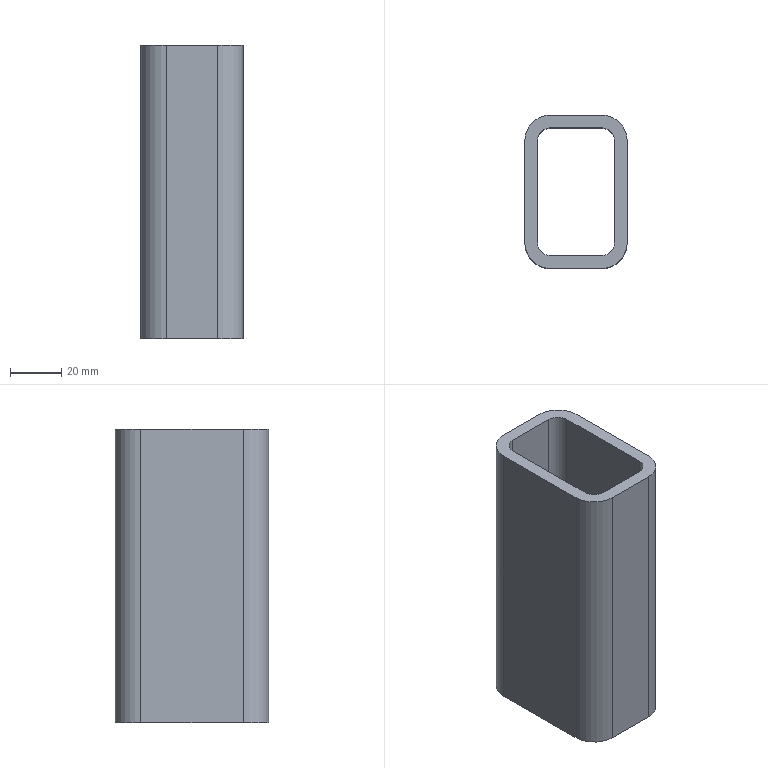Part | STEP file | HL4GD-1.30.113 base frame front support vertical beam--20251212 | 1 solid | 18 faces | box 40 x 60 x 115 mm | volume 96096 mm3 | plane 10 | cylinder 8 | commonest cylinder face diameters 10 x4 20 x4
STEP:
#1=CARTESIAN_POINT('',(0.,0.,0.));
#2=DIRECTION('',(0.,0.,1.));
#3=DIRECTION('',(1.,0.,0.));
#4=AXIS2_PLACEMENT_3D('',#1,#2,#3);
#5=CARTESIAN_POINT('',(2870.,610.,405.));
#6=VERTEX_POINT('',#5);
#7=CARTESIAN_POINT('',(2875.,615.,405.));
#8=VERTEX_POINT('',#7);
#9=CARTESIAN_POINT('',(2875.,610.,405.));
#10=DIRECTION('',(0.,0.,-1.));
#11=DIRECTION('',(0.,1.,0.));
#12=AXIS2_PLACEMENT_3D('',#9,#10,#11);
#13=CIRCLE('',#12,5.);
#14=CARTESIAN_POINT('',(2875.,610.,1349.));
#15=DIRECTION('',(0.,0.,1.));
#16=DIRECTION('',(-1.,0.,0.));
#17=AXIS2_PLACEMENT_3D('',#14,#15,#16);
#18=CYLINDRICAL_SURFACE('',#17,5.);
#19=CARTESIAN_POINT('',(10.996,-944.));
#20=DIRECTION('',(-1.,0.));
#21=VECTOR('',#20,1.);
#22=LINE('',#19,#21);
#23=(GEOMETRIC_REPRESENTATION_CONTEXT(2)PARAMETRIC_REPRESENTATION_CONTEXT()REPRESENTATION_CONTEXT('',''));
#24=DEFINITIONAL_REPRESENTATION('',(#22),#23);
#25=PCURVE('',#18,#24);
#26=CARTESIAN_POINT('',(2885.,1185.,405.));
#27=DIRECTION('',(0.,0.,1.));
#28=DIRECTION('',(0.,1.,0.));
#29=AXIS2_PLACEMENT_3D('',#26,#27,#28);
#30=PLANE('',#29);
#31=CARTESIAN_POINT('',(-570.,10.));
#32=CARTESIAN_POINT('',(-570.,1.34));
#33=CARTESIAN_POINT('',(-577.5,5.67));
#34=CARTESIAN_POINT('',(-585.,10.));
#35=CARTESIAN_POINT('',(-577.5,14.33));
#36=CARTESIAN_POINT('',(-570.,18.66));
#37=CARTESIAN_POINT('',(-570.,10.));
#38=(BOUNDED_CURVE()B_SPLINE_CURVE(2,(#31,#32,#33,#34,#35,#36,#37),.UNSPECIFIED.,.T.,.F.)B_SPLINE_CURVE_WITH_KNOTS((1,2,2,2,2,1),(-2.094,0.,2.094,4.189,6.283,8.378),.UNSPECIFIED.)CURVE()GEOMETRIC_REPRESENTATION_ITEM()RATIONAL_B_SPLINE_CURVE((1.,0.5,1.,0.5,1.,0.5,1.))REPRESENTATION_ITEM(''));
#39=(GEOMETRIC_REPRESENTATION_CONTEXT(2)PARAMETRIC_REPRESENTATION_CONTEXT()REPRESENTATION_CONTEXT('',''));
#40=DEFINITIONAL_REPRESENTATION('',(#38),#39);
#41=PCURVE('',#30,#40);
#42=SURFACE_CURVE('',#13,(#25,#41),.PCURVE_S1.);
#43=EDGE_CURVE('',#6,#8,#42,.T.);
#44=ORIENTED_EDGE('',*,*,#43,.F.);
#45=CARTESIAN_POINT('',(2870.,610.,520.));
#46=VERTEX_POINT('',#45);
#47=CARTESIAN_POINT('',(2870.,610.,1349.));
#48=DIRECTION('',(0.,0.,1.));
#49=VECTOR('',#48,1.);
#50=LINE('',#47,#49);
#51=CARTESIAN_POINT('',(6.283,0.));
#52=DIRECTION('',(0.,1.));
#53=VECTOR('',#52,1.);
#54=LINE('',#51,#53);
#55=(GEOMETRIC_REPRESENTATION_CONTEXT(2)PARAMETRIC_REPRESENTATION_CONTEXT()REPRESENTATION_CONTEXT('',''));
#56=DEFINITIONAL_REPRESENTATION('',(#54),#55);
#57=PCURVE('',#18,#56);
#58=CARTESIAN_POINT('',(2870.,610.,1349.));
#59=DIRECTION('',(1.,0.,0.));
#60=DIRECTION('',(0.,1.,0.));
#61=AXIS2_PLACEMENT_3D('',#58,#59,#60);
#62=PLANE('',#61);
#63=CARTESIAN_POINT('',(0.,0.));
#64=DIRECTION('',(0.,1.));
#65=VECTOR('',#64,1.);
#66=LINE('',#63,#65);
#67=(GEOMETRIC_REPRESENTATION_CONTEXT(2)PARAMETRIC_REPRESENTATION_CONTEXT()REPRESENTATION_CONTEXT('',''));
#68=DEFINITIONAL_REPRESENTATION('',(#66),#67);
#69=PCURVE('',#62,#68);
#70=SURFACE_CURVE('',#50,(#57,#69),.PCURVE_S1.);
#71=EDGE_CURVE('',#6,#46,#70,.T.);
#72=ORIENTED_EDGE('',*,*,#71,.T.);
#73=CARTESIAN_POINT('',(2875.,615.,520.));
#74=VERTEX_POINT('',#73);
#75=CARTESIAN_POINT('',(2875.,610.,520.));
#76=DIRECTION('',(0.,0.,1.));
#77=DIRECTION('',(1.,0.,0.));
#78=AXIS2_PLACEMENT_3D('',#75,#76,#77);
#79=CIRCLE('',#78,5.);
#80=CARTESIAN_POINT('',(3.142,-829.));
#81=DIRECTION('',(1.,0.));
#82=VECTOR('',#81,1.);
#83=LINE('',#80,#82);
#84=(GEOMETRIC_REPRESENTATION_CONTEXT(2)PARAMETRIC_REPRESENTATION_CONTEXT()REPRESENTATION_CONTEXT('',''));
#85=DEFINITIONAL_REPRESENTATION('',(#83),#84);
#86=PCURVE('',#18,#85);
#87=CARTESIAN_POINT('',(2455.,590.,520.));
#88=DIRECTION('',(0.,0.,1.));
#89=DIRECTION('',(1.,0.,0.));
#90=AXIS2_PLACEMENT_3D('',#87,#88,#89);
#91=PLANE('',#90);
#92=CARTESIAN_POINT('',(420.,20.));
#93=DIRECTION('',(1.,0.));
#94=AXIS2_PLACEMENT_2D('',#92,#93);
#95=CIRCLE('',#94,5.);
#96=(GEOMETRIC_REPRESENTATION_CONTEXT(2)PARAMETRIC_REPRESENTATION_CONTEXT()REPRESENTATION_CONTEXT('',''));
#97=DEFINITIONAL_REPRESENTATION('',(#95),#96);
#98=PCURVE('',#91,#97);
#99=SURFACE_CURVE('',#79,(#86,#98),.PCURVE_S1.);
#100=EDGE_CURVE('',#74,#46,#99,.T.);
#101=ORIENTED_EDGE('',*,*,#100,.F.);
#102=CARTESIAN_POINT('',(2875.,615.,1349.));
#103=DIRECTION('',(0.,0.,1.));
#104=VECTOR('',#103,1.);
#105=LINE('',#102,#104);
#106=CARTESIAN_POINT('',(4.712,0.));
#107=DIRECTION('',(0.,1.));
#108=VECTOR('',#107,1.);
#109=LINE('',#106,#108);
#110=(GEOMETRIC_REPRESENTATION_CONTEXT(2)PARAMETRIC_REPRESENTATION_CONTEXT()REPRESENTATION_CONTEXT('',''));
#111=DEFINITIONAL_REPRESENTATION('',(#109),#110);
#112=PCURVE('',#18,#111);
#113=CARTESIAN_POINT('',(2895.,615.,1349.));
#114=DIRECTION('',(0.,-1.,0.));
#115=DIRECTION('',(1.,0.,0.));
#116=AXIS2_PLACEMENT_3D('',#113,#114,#115);
#117=PLANE('',#116);
#118=CARTESIAN_POINT('',(-20.,0.));
#119=DIRECTION('',(0.,1.));
#120=VECTOR('',#119,1.);
#121=LINE('',#118,#120);
#122=(GEOMETRIC_REPRESENTATION_CONTEXT(2)PARAMETRIC_REPRESENTATION_CONTEXT()REPRESENTATION_CONTEXT('',''));
#123=DEFINITIONAL_REPRESENTATION('',(#121),#122);
#124=PCURVE('',#117,#123);
#125=SURFACE_CURVE('',#105,(#112,#124),.PCURVE_S1.);
#126=EDGE_CURVE('',#8,#74,#125,.T.);
#127=ORIENTED_EDGE('',*,*,#126,.F.);
#128=EDGE_LOOP('',(#44,#72,#101,#127));
#129=FACE_BOUND('',#128,.F.);
#130=ADVANCED_FACE('',(#129),#18,.F.);
#131=CARTESIAN_POINT('',(2895.,615.,405.));
#132=VERTEX_POINT('',#131);
#133=CARTESIAN_POINT('',(2895.,615.,520.));
#134=VERTEX_POINT('',#133);
#135=CARTESIAN_POINT('',(2895.,615.,1349.));
#136=DIRECTION('',(0.,0.,1.));
#137=VECTOR('',#136,1.);
#138=LINE('',#135,#137);
#139=CARTESIAN_POINT('',(0.,0.));
#140=DIRECTION('',(0.,1.));
#141=VECTOR('',#140,1.);
#142=LINE('',#139,#141);
#143=(GEOMETRIC_REPRESENTATION_CONTEXT(2)PARAMETRIC_REPRESENTATION_CONTEXT()REPRESENTATION_CONTEXT('',''));
#144=DEFINITIONAL_REPRESENTATION('',(#142),#143);
#145=PCURVE('',#117,#144);
#146=CARTESIAN_POINT('',(2895.,610.,1349.));
#147=DIRECTION('',(0.,0.,1.));
#148=DIRECTION('',(-1.,0.,0.));
#149=AXIS2_PLACEMENT_3D('',#146,#147,#148);
#150=CYLINDRICAL_SURFACE('',#149,5.);
#151=CARTESIAN_POINT('',(4.712,0.));
#152=DIRECTION('',(0.,1.));
#153=VECTOR('',#152,1.);
#154=LINE('',#151,#153);
#155=(GEOMETRIC_REPRESENTATION_CONTEXT(2)PARAMETRIC_REPRESENTATION_CONTEXT()REPRESENTATION_CONTEXT('',''));
#156=DEFINITIONAL_REPRESENTATION('',(#154),#155);
#157=PCURVE('',#150,#156);
#158=SURFACE_CURVE('',#138,(#145,#157),.PCURVE_S1.);
#159=EDGE_CURVE('',#132,#134,#158,.T.);
#160=ORIENTED_EDGE('',*,*,#159,.T.);
#161=CARTESIAN_POINT('',(2895.,615.,520.));
#162=DIRECTION('',(-1.,0.,0.));
#163=VECTOR('',#162,1.);
#164=LINE('',#161,#163);
#165=CARTESIAN_POINT('',(0.,-829.));
#166=DIRECTION('',(-1.,0.));
#167=VECTOR('',#166,1.);
#168=LINE('',#165,#167);
#169=(GEOMETRIC_REPRESENTATION_CONTEXT(2)PARAMETRIC_REPRESENTATION_CONTEXT()REPRESENTATION_CONTEXT('',''));
#170=DEFINITIONAL_REPRESENTATION('',(#168),#169);
#171=PCURVE('',#117,#170);
#172=CARTESIAN_POINT('',(440.,25.));
#173=DIRECTION('',(-1.,0.));
#174=VECTOR('',#173,1.);
#175=LINE('',#172,#174);
#176=(GEOMETRIC_REPRESENTATION_CONTEXT(2)PARAMETRIC_REPRESENTATION_CONTEXT()REPRESENTATION_CONTEXT('',''));
#177=DEFINITIONAL_REPRESENTATION('',(#175),#176);
#178=PCURVE('',#91,#177);
#179=SURFACE_CURVE('',#164,(#171,#178),.PCURVE_S1.);
#180=EDGE_CURVE('',#134,#74,#179,.T.);
#181=ORIENTED_EDGE('',*,*,#180,.T.);
#182=ORIENTED_EDGE('',*,*,#126,.F.);
#183=CARTESIAN_POINT('',(2895.,615.,405.));
#184=DIRECTION('',(1.,0.,0.));
#185=VECTOR('',#184,1.);
#186=LINE('',#183,#185);
#187=CARTESIAN_POINT('',(0.,-944.));
#188=DIRECTION('',(1.,0.));
#189=VECTOR('',#188,1.);
#190=LINE('',#187,#189);
#191=(GEOMETRIC_REPRESENTATION_CONTEXT(2)PARAMETRIC_REPRESENTATION_CONTEXT()REPRESENTATION_CONTEXT('',''));
#192=DEFINITIONAL_REPRESENTATION('',(#190),#191);
#193=PCURVE('',#117,#192);
#194=CARTESIAN_POINT('',(-570.,-10.));
#195=DIRECTION('',(0.,-1.));
#196=VECTOR('',#195,1.);
#197=LINE('',#194,#196);
#198=(GEOMETRIC_REPRESENTATION_CONTEXT(2)PARAMETRIC_REPRESENTATION_CONTEXT()REPRESENTATION_CONTEXT('',''));
#199=DEFINITIONAL_REPRESENTATION('',(#197),#198);
#200=PCURVE('',#30,#199);
#201=SURFACE_CURVE('',#186,(#193,#200),.PCURVE_S1.);
#202=EDGE_CURVE('',#8,#132,#201,.T.);
#203=ORIENTED_EDGE('',*,*,#202,.T.);
#204=EDGE_LOOP('',(#160,#181,#182,#203));
#205=FACE_BOUND('',#204,.T.);
#206=ADVANCED_FACE('',(#205),#117,.T.);
#207=CARTESIAN_POINT('',(2900.,610.,405.));
#208=VERTEX_POINT('',#207);
#209=CARTESIAN_POINT('',(2895.,610.,405.));
#210=DIRECTION('',(0.,0.,1.));
#211=DIRECTION('',(0.,1.,0.));
#212=AXIS2_PLACEMENT_3D('',#209,#210,#211);
#213=CIRCLE('',#212,5.);
#214=CARTESIAN_POINT('',(-1.571,-944.));
#215=DIRECTION('',(1.,0.));
#216=VECTOR('',#215,1.);
#217=LINE('',#214,#216);
#218=(GEOMETRIC_REPRESENTATION_CONTEXT(2)PARAMETRIC_REPRESENTATION_CONTEXT()REPRESENTATION_CONTEXT('',''));
#219=DEFINITIONAL_REPRESENTATION('',(#217),#218);
#220=PCURVE('',#150,#219);
#221=CARTESIAN_POINT('',(-575.,-10.));
#222=DIRECTION('',(1.,0.));
#223=AXIS2_PLACEMENT_2D('',#221,#222);
#224=CIRCLE('',#223,5.);
#225=(GEOMETRIC_REPRESENTATION_CONTEXT(2)PARAMETRIC_REPRESENTATION_CONTEXT()REPRESENTATION_CONTEXT('',''));
#226=DEFINITIONAL_REPRESENTATION('',(#224),#225);
#227=PCURVE('',#30,#226);
#228=SURFACE_CURVE('',#213,(#220,#227),.PCURVE_S1.);
#229=EDGE_CURVE('',#208,#132,#228,.T.);
#230=ORIENTED_EDGE('',*,*,#229,.T.);
#231=ORIENTED_EDGE('',*,*,#159,.T.);
#232=CARTESIAN_POINT('',(2900.,610.,520.));
#233=VERTEX_POINT('',#232);
#234=CARTESIAN_POINT('',(2895.,610.,520.));
#235=DIRECTION('',(0.,0.,1.));
#236=DIRECTION('',(1.,0.,0.));
#237=AXIS2_PLACEMENT_3D('',#234,#235,#236);
#238=CIRCLE('',#237,5.);
#239=CARTESIAN_POINT('',(3.142,-829.));
#240=DIRECTION('',(1.,0.));
#241=VECTOR('',#240,1.);
#242=LINE('',#239,#241);
#243=(GEOMETRIC_REPRESENTATION_CONTEXT(2)PARAMETRIC_REPRESENTATION_CONTEXT()REPRESENTATION_CONTEXT('',''));
#244=DEFINITIONAL_REPRESENTATION('',(#242),#243);
#245=PCURVE('',#150,#244);
#246=CARTESIAN_POINT('',(440.,20.));
#247=DIRECTION('',(1.,0.));
#248=AXIS2_PLACEMENT_2D('',#246,#247);
#249=CIRCLE('',#248,5.);
#250=(GEOMETRIC_REPRESENTATION_CONTEXT(2)PARAMETRIC_REPRESENTATION_CONTEXT()REPRESENTATION_CONTEXT('',''));
#251=DEFINITIONAL_REPRESENTATION('',(#249),#250);
#252=PCURVE('',#91,#251);
#253=SURFACE_CURVE('',#238,(#245,#252),.PCURVE_S1.);
#254=EDGE_CURVE('',#233,#134,#253,.T.);
#255=ORIENTED_EDGE('',*,*,#254,.F.);
#256=CARTESIAN_POINT('',(2900.,610.,1349.));
#257=DIRECTION('',(0.,0.,1.));
#258=VECTOR('',#257,1.);
#259=LINE('',#256,#258);
#260=CARTESIAN_POINT('',(3.142,0.));
#261=DIRECTION('',(0.,1.));
#262=VECTOR('',#261,1.);
#263=LINE('',#260,#262);
#264=(GEOMETRIC_REPRESENTATION_CONTEXT(2)PARAMETRIC_REPRESENTATION_CONTEXT()REPRESENTATION_CONTEXT('',''));
#265=DEFINITIONAL_REPRESENTATION('',(#263),#264);
#266=PCURVE('',#150,#265);
#267=CARTESIAN_POINT('',(2900.,570.,1349.));
#268=DIRECTION('',(-1.,0.,0.));
#269=DIRECTION('',(0.,-1.,0.));
#270=AXIS2_PLACEMENT_3D('',#267,#268,#269);
#271=PLANE('',#270);
#272=CARTESIAN_POINT('',(-40.,0.));
#273=DIRECTION('',(0.,1.));
#274=VECTOR('',#273,1.);
#275=LINE('',#272,#274);
#276=(GEOMETRIC_REPRESENTATION_CONTEXT(2)PARAMETRIC_REPRESENTATION_CONTEXT()REPRESENTATION_CONTEXT('',''));
#277=DEFINITIONAL_REPRESENTATION('',(#275),#276);
#278=PCURVE('',#271,#277);
#279=SURFACE_CURVE('',#259,(#266,#278),.PCURVE_S1.);
#280=EDGE_CURVE('',#208,#233,#279,.T.);
#281=ORIENTED_EDGE('',*,*,#280,.F.);
#282=EDGE_LOOP('',(#230,#231,#255,#281));
#283=FACE_BOUND('',#282,.F.);
#284=ADVANCED_FACE('',(#283),#150,.F.);
#285=CARTESIAN_POINT('',(2900.,570.,405.));
#286=VERTEX_POINT('',#285);
#287=CARTESIAN_POINT('',(2900.,570.,520.));
#288=VERTEX_POINT('',#287);
#289=CARTESIAN_POINT('',(2900.,570.,1349.));
#290=DIRECTION('',(0.,0.,1.));
#291=VECTOR('',#290,1.);
#292=LINE('',#289,#291);
#293=CARTESIAN_POINT('',(0.,0.));
#294=DIRECTION('',(0.,1.));
#295=VECTOR('',#294,1.);
#296=LINE('',#293,#295);
#297=(GEOMETRIC_REPRESENTATION_CONTEXT(2)PARAMETRIC_REPRESENTATION_CONTEXT()REPRESENTATION_CONTEXT('',''));
#298=DEFINITIONAL_REPRESENTATION('',(#296),#297);
#299=PCURVE('',#271,#298);
#300=CARTESIAN_POINT('',(2895.,570.,1349.));
#301=DIRECTION('',(0.,0.,1.));
#302=DIRECTION('',(-1.,0.,0.));
#303=AXIS2_PLACEMENT_3D('',#300,#301,#302);
#304=CYLINDRICAL_SURFACE('',#303,5.);
#305=CARTESIAN_POINT('',(3.142,0.));
#306=DIRECTION('',(0.,1.));
#307=VECTOR('',#306,1.);
#308=LINE('',#305,#307);
#309=(GEOMETRIC_REPRESENTATION_CONTEXT(2)PARAMETRIC_REPRESENTATION_CONTEXT()REPRESENTATION_CONTEXT('',''));
#310=DEFINITIONAL_REPRESENTATION('',(#308),#309);
#311=PCURVE('',#304,#310);
#312=SURFACE_CURVE('',#292,(#299,#311),.PCURVE_S1.);
#313=EDGE_CURVE('',#286,#288,#312,.T.);
#314=ORIENTED_EDGE('',*,*,#313,.T.);
#315=CARTESIAN_POINT('',(2900.,570.,520.));
#316=DIRECTION('',(0.,1.,0.));
#317=VECTOR('',#316,1.);
#318=LINE('',#315,#317);
#319=CARTESIAN_POINT('',(0.,-829.));
#320=DIRECTION('',(-1.,0.));
#321=VECTOR('',#320,1.);
#322=LINE('',#319,#321);
#323=(GEOMETRIC_REPRESENTATION_CONTEXT(2)PARAMETRIC_REPRESENTATION_CONTEXT()REPRESENTATION_CONTEXT('',''));
#324=DEFINITIONAL_REPRESENTATION('',(#322),#323);
#325=PCURVE('',#271,#324);
#326=CARTESIAN_POINT('',(445.,-20.));
#327=DIRECTION('',(0.,1.));
#328=VECTOR('',#327,1.);
#329=LINE('',#326,#328);
#330=(GEOMETRIC_REPRESENTATION_CONTEXT(2)PARAMETRIC_REPRESENTATION_CONTEXT()REPRESENTATION_CONTEXT('',''));
#331=DEFINITIONAL_REPRESENTATION('',(#329),#330);
#332=PCURVE('',#91,#331);
#333=SURFACE_CURVE('',#318,(#325,#332),.PCURVE_S1.);
#334=EDGE_CURVE('',#288,#233,#333,.T.);
#335=ORIENTED_EDGE('',*,*,#334,.T.);
#336=ORIENTED_EDGE('',*,*,#280,.F.);
#337=CARTESIAN_POINT('',(2900.,570.,405.));
#338=DIRECTION('',(0.,1.,0.));
#339=VECTOR('',#338,1.);
#340=LINE('',#337,#339);
#341=CARTESIAN_POINT('',(0.,-944.));
#342=DIRECTION('',(-1.,0.));
#343=VECTOR('',#342,1.);
#344=LINE('',#341,#343);
#345=(GEOMETRIC_REPRESENTATION_CONTEXT(2)PARAMETRIC_REPRESENTATION_CONTEXT()REPRESENTATION_CONTEXT('',''));
#346=DEFINITIONAL_REPRESENTATION('',(#344),#345);
#347=PCURVE('',#271,#346);
#348=CARTESIAN_POINT('',(-615.,-15.));
#349=DIRECTION('',(1.,0.));
#350=VECTOR('',#349,1.);
#351=LINE('',#348,#350);
#352=(GEOMETRIC_REPRESENTATION_CONTEXT(2)PARAMETRIC_REPRESENTATION_CONTEXT()REPRESENTATION_CONTEXT('',''));
#353=DEFINITIONAL_REPRESENTATION('',(#351),#352);
#354=PCURVE('',#30,#353);
#355=SURFACE_CURVE('',#340,(#347,#354),.PCURVE_S1.);
#356=EDGE_CURVE('',#286,#208,#355,.T.);
#357=ORIENTED_EDGE('',*,*,#356,.F.);
#358=EDGE_LOOP('',(#314,#335,#336,#357));
#359=FACE_BOUND('',#358,.T.);
#360=ADVANCED_FACE('',(#359),#271,.T.);
#361=CARTESIAN_POINT('',(2895.,565.,405.));
#362=VERTEX_POINT('',#361);
#363=CARTESIAN_POINT('',(2895.,570.,405.));
#364=DIRECTION('',(0.,0.,1.));
#365=DIRECTION('',(0.,1.,0.));
#366=AXIS2_PLACEMENT_3D('',#363,#364,#365);
#367=CIRCLE('',#366,5.);
#368=CARTESIAN_POINT('',(-1.571,-944.));
#369=DIRECTION('',(1.,0.));
#370=VECTOR('',#369,1.);
#371=LINE('',#368,#370);
#372=(GEOMETRIC_REPRESENTATION_CONTEXT(2)PARAMETRIC_REPRESENTATION_CONTEXT()REPRESENTATION_CONTEXT('',''));
#373=DEFINITIONAL_REPRESENTATION('',(#371),#372);
#374=PCURVE('',#304,#373);
#375=CARTESIAN_POINT('',(-615.,-10.));
#376=DIRECTION('',(1.,0.));
#377=AXIS2_PLACEMENT_2D('',#375,#376);
#378=CIRCLE('',#377,5.);
#379=(GEOMETRIC_REPRESENTATION_CONTEXT(2)PARAMETRIC_REPRESENTATION_CONTEXT()REPRESENTATION_CONTEXT('',''));
#380=DEFINITIONAL_REPRESENTATION('',(#378),#379);
#381=PCURVE('',#30,#380);
#382=SURFACE_CURVE('',#367,(#374,#381),.PCURVE_S1.);
#383=EDGE_CURVE('',#362,#286,#382,.T.);
#384=ORIENTED_EDGE('',*,*,#383,.T.);
#385=ORIENTED_EDGE('',*,*,#313,.T.);
#386=CARTESIAN_POINT('',(2895.,565.,520.));
#387=VERTEX_POINT('',#386);
#388=CARTESIAN_POINT('',(2895.,570.,520.));
#389=DIRECTION('',(0.,0.,1.));
#390=DIRECTION('',(1.,0.,0.));
#391=AXIS2_PLACEMENT_3D('',#388,#389,#390);
#392=CIRCLE('',#391,5.);
#393=CARTESIAN_POINT('',(-3.142,-829.));
#394=DIRECTION('',(1.,0.));
#395=VECTOR('',#394,1.);
#396=LINE('',#393,#395);
#397=(GEOMETRIC_REPRESENTATION_CONTEXT(2)PARAMETRIC_REPRESENTATION_CONTEXT()REPRESENTATION_CONTEXT('',''));
#398=DEFINITIONAL_REPRESENTATION('',(#396),#397);
#399=PCURVE('',#304,#398);
#400=CARTESIAN_POINT('',(440.,-20.));
#401=DIRECTION('',(1.,0.));
#402=AXIS2_PLACEMENT_2D('',#400,#401);
#403=CIRCLE('',#402,5.);
#404=(GEOMETRIC_REPRESENTATION_CONTEXT(2)PARAMETRIC_REPRESENTATION_CONTEXT()REPRESENTATION_CONTEXT('',''));
#405=DEFINITIONAL_REPRESENTATION('',(#403),#404);
#406=PCURVE('',#91,#405);
#407=SURFACE_CURVE('',#392,(#399,#406),.PCURVE_S1.);
#408=EDGE_CURVE('',#387,#288,#407,.T.);
#409=ORIENTED_EDGE('',*,*,#408,.F.);
#410=CARTESIAN_POINT('',(2895.,565.,1349.));
#411=DIRECTION('',(0.,0.,1.));
#412=VECTOR('',#411,1.);
#413=LINE('',#410,#412);
#414=CARTESIAN_POINT('',(1.571,0.));
#415=DIRECTION('',(0.,1.));
#416=VECTOR('',#415,1.);
#417=LINE('',#414,#416);
#418=(GEOMETRIC_REPRESENTATION_CONTEXT(2)PARAMETRIC_REPRESENTATION_CONTEXT()REPRESENTATION_CONTEXT('',''));
#419=DEFINITIONAL_REPRESENTATION('',(#417),#418);
#420=PCURVE('',#304,#419);
#421=CARTESIAN_POINT('',(2875.,565.,1349.));
#422=DIRECTION('',(0.,1.,0.));
#423=DIRECTION('',(-1.,0.,0.));
#424=AXIS2_PLACEMENT_3D('',#421,#422,#423);
#425=PLANE('',#424);
#426=CARTESIAN_POINT('',(-20.,0.));
#427=DIRECTION('',(0.,1.));
#428=VECTOR('',#427,1.);
#429=LINE('',#426,#428);
#430=(GEOMETRIC_REPRESENTATION_CONTEXT(2)PARAMETRIC_REPRESENTATION_CONTEXT()REPRESENTATION_CONTEXT('',''));
#431=DEFINITIONAL_REPRESENTATION('',(#429),#430);
#432=PCURVE('',#425,#431);
#433=SURFACE_CURVE('',#413,(#420,#432),.PCURVE_S1.);
#434=EDGE_CURVE('',#362,#387,#433,.T.);
#435=ORIENTED_EDGE('',*,*,#434,.F.);
#436=EDGE_LOOP('',(#384,#385,#409,#435));
#437=FACE_BOUND('',#436,.F.);
#438=ADVANCED_FACE('',(#437),#304,.F.);
#439=CARTESIAN_POINT('',(2875.,565.,405.));
#440=VERTEX_POINT('',#439);
#441=CARTESIAN_POINT('',(2875.,565.,520.));
#442=VERTEX_POINT('',#441);
#443=CARTESIAN_POINT('',(2875.,565.,1349.));
#444=DIRECTION('',(0.,0.,1.));
#445=VECTOR('',#444,1.);
#446=LINE('',#443,#445);
#447=CARTESIAN_POINT('',(0.,0.));
#448=DIRECTION('',(0.,1.));
#449=VECTOR('',#448,1.);
#450=LINE('',#447,#449);
#451=(GEOMETRIC_REPRESENTATION_CONTEXT(2)PARAMETRIC_REPRESENTATION_CONTEXT()REPRESENTATION_CONTEXT('',''));
#452=DEFINITIONAL_REPRESENTATION('',(#450),#451);
#453=PCURVE('',#425,#452);
#454=CARTESIAN_POINT('',(2875.,570.,1349.));
#455=DIRECTION('',(0.,0.,1.));
#456=DIRECTION('',(-1.,0.,0.));
#457=AXIS2_PLACEMENT_3D('',#454,#455,#456);
#458=CYLINDRICAL_SURFACE('',#457,5.);
#459=CARTESIAN_POINT('',(1.571,0.));
#460=DIRECTION('',(0.,1.));
#461=VECTOR('',#460,1.);
#462=LINE('',#459,#461);
#463=(GEOMETRIC_REPRESENTATION_CONTEXT(2)PARAMETRIC_REPRESENTATION_CONTEXT()REPRESENTATION_CONTEXT('',''));
#464=DEFINITIONAL_REPRESENTATION('',(#462),#463);
#465=PCURVE('',#458,#464);
#466=SURFACE_CURVE('',#446,(#453,#465),.PCURVE_S1.);
#467=EDGE_CURVE('',#440,#442,#466,.T.);
#468=ORIENTED_EDGE('',*,*,#467,.T.);
#469=CARTESIAN_POINT('',(2875.,565.,520.));
#470=DIRECTION('',(1.,0.,0.));
#471=VECTOR('',#470,1.);
#472=LINE('',#469,#471);
#473=CARTESIAN_POINT('',(0.,-829.));
#474=DIRECTION('',(-1.,0.));
#475=VECTOR('',#474,1.);
#476=LINE('',#473,#475);
#477=(GEOMETRIC_REPRESENTATION_CONTEXT(2)PARAMETRIC_REPRESENTATION_CONTEXT()REPRESENTATION_CONTEXT('',''));
#478=DEFINITIONAL_REPRESENTATION('',(#476),#477);
#479=PCURVE('',#425,#478);
#480=CARTESIAN_POINT('',(420.,-25.));
#481=DIRECTION('',(1.,0.));
#482=VECTOR('',#481,1.);
#483=LINE('',#480,#482);
#484=(GEOMETRIC_REPRESENTATION_CONTEXT(2)PARAMETRIC_REPRESENTATION_CONTEXT()REPRESENTATION_CONTEXT('',''));
#485=DEFINITIONAL_REPRESENTATION('',(#483),#484);
#486=PCURVE('',#91,#485);
#487=SURFACE_CURVE('',#472,(#479,#486),.PCURVE_S1.);
#488=EDGE_CURVE('',#442,#387,#487,.T.);
#489=ORIENTED_EDGE('',*,*,#488,.T.);
#490=ORIENTED_EDGE('',*,*,#434,.F.);
#491=CARTESIAN_POINT('',(2875.,565.,405.));
#492=DIRECTION('',(1.,0.,0.));
#493=VECTOR('',#492,1.);
#494=LINE('',#491,#493);
#495=CARTESIAN_POINT('',(0.,-944.));
#496=DIRECTION('',(-1.,0.));
#497=VECTOR('',#496,1.);
#498=LINE('',#495,#497);
#499=(GEOMETRIC_REPRESENTATION_CONTEXT(2)PARAMETRIC_REPRESENTATION_CONTEXT()REPRESENTATION_CONTEXT('',''));
#500=DEFINITIONAL_REPRESENTATION('',(#498),#499);
#501=PCURVE('',#425,#500);
#502=CARTESIAN_POINT('',(-620.,10.));
#503=DIRECTION('',(0.,-1.));
#504=VECTOR('',#503,1.);
#505=LINE('',#502,#504);
#506=(GEOMETRIC_REPRESENTATION_CONTEXT(2)PARAMETRIC_REPRESENTATION_CONTEXT()REPRESENTATION_CONTEXT('',''));
#507=DEFINITIONAL_REPRESENTATION('',(#505),#506);
#508=PCURVE('',#30,#507);
#509=SURFACE_CURVE('',#494,(#501,#508),.PCURVE_S1.);
#510=EDGE_CURVE('',#440,#362,#509,.T.);
#511=ORIENTED_EDGE('',*,*,#510,.F.);
#512=EDGE_LOOP('',(#468,#489,#490,#511));
#513=FACE_BOUND('',#512,.T.);
#514=ADVANCED_FACE('',(#513),#425,.T.);
#515=CARTESIAN_POINT('',(2870.,570.,405.));
#516=VERTEX_POINT('',#515);
#517=CARTESIAN_POINT('',(2875.,570.,405.));
#518=DIRECTION('',(0.,0.,-1.));
#519=DIRECTION('',(0.,1.,0.));
#520=AXIS2_PLACEMENT_3D('',#517,#518,#519);
#521=CIRCLE('',#520,5.);
#522=CARTESIAN_POINT('',(4.712,-944.));
#523=DIRECTION('',(-1.,0.));
#524=VECTOR('',#523,1.);
#525=LINE('',#522,#524);
#526=(GEOMETRIC_REPRESENTATION_CONTEXT(2)PARAMETRIC_REPRESENTATION_CONTEXT()REPRESENTATION_CONTEXT('',''));
#527=DEFINITIONAL_REPRESENTATION('',(#525),#526);
#528=PCURVE('',#458,#527);
#529=CARTESIAN_POINT('',(-610.,10.));
#530=CARTESIAN_POINT('',(-610.,1.34));
#531=CARTESIAN_POINT('',(-617.5,5.67));
#532=CARTESIAN_POINT('',(-625.,10.));
#533=CARTESIAN_POINT('',(-617.5,14.33));
#534=CARTESIAN_POINT('',(-610.,18.66));
#535=CARTESIAN_POINT('',(-610.,10.));
#536=(BOUNDED_CURVE()B_SPLINE_CURVE(2,(#529,#530,#531,#532,#533,#534,#535),.UNSPECIFIED.,.T.,.F.)B_SPLINE_CURVE_WITH_KNOTS((1,2,2,2,2,1),(-2.094,0.,2.094,4.189,6.283,8.378),.UNSPECIFIED.)CURVE()GEOMETRIC_REPRESENTATION_ITEM()RATIONAL_B_SPLINE_CURVE((1.,0.5,1.,0.5,1.,0.5,1.))REPRESENTATION_ITEM(''));
#537=(GEOMETRIC_REPRESENTATION_CONTEXT(2)PARAMETRIC_REPRESENTATION_CONTEXT()REPRESENTATION_CONTEXT('',''));
#538=DEFINITIONAL_REPRESENTATION('',(#536),#537);
#539=PCURVE('',#30,#538);
#540=SURFACE_CURVE('',#521,(#528,#539),.PCURVE_S1.);
#541=EDGE_CURVE('',#440,#516,#540,.T.);
#542=ORIENTED_EDGE('',*,*,#541,.F.);
#543=ORIENTED_EDGE('',*,*,#467,.T.);
#544=CARTESIAN_POINT('',(2870.,570.,520.));
#545=VERTEX_POINT('',#544);
#546=CARTESIAN_POINT('',(2875.,570.,520.));
#547=DIRECTION('',(0.,0.,1.));
#548=DIRECTION('',(1.,0.,0.));
#549=AXIS2_PLACEMENT_3D('',#546,#547,#548);
#550=CIRCLE('',#549,5.);
#551=CARTESIAN_POINT('',(-3.142,-829.));
#552=DIRECTION('',(1.,0.));
#553=VECTOR('',#552,1.);
#554=LINE('',#551,#553);
#555=(GEOMETRIC_REPRESENTATION_CONTEXT(2)PARAMETRIC_REPRESENTATION_CONTEXT()REPRESENTATION_CONTEXT('',''));
#556=DEFINITIONAL_REPRESENTATION('',(#554),#555);
#557=PCURVE('',#458,#556);
#558=CARTESIAN_POINT('',(420.,-20.));
#559=DIRECTION('',(1.,0.));
#560=AXIS2_PLACEMENT_2D('',#558,#559);
#561=CIRCLE('',#560,5.);
#562=(GEOMETRIC_REPRESENTATION_CONTEXT(2)PARAMETRIC_REPRESENTATION_CONTEXT()REPRESENTATION_CONTEXT('',''));
#563=DEFINITIONAL_REPRESENTATION('',(#561),#562);
#564=PCURVE('',#91,#563);
#565=SURFACE_CURVE('',#550,(#557,#564),.PCURVE_S1.);
#566=EDGE_CURVE('',#545,#442,#565,.T.);
#567=ORIENTED_EDGE('',*,*,#566,.F.);
#568=CARTESIAN_POINT('',(2870.,570.,1349.));
#569=DIRECTION('',(0.,0.,1.));
#570=VECTOR('',#569,1.);
#571=LINE('',#568,#570);
#572=CARTESIAN_POINT('',(0.,0.));
#573=DIRECTION('',(0.,1.));
#574=VECTOR('',#573,1.);
#575=LINE('',#572,#574);
#576=(GEOMETRIC_REPRESENTATION_CONTEXT(2)PARAMETRIC_REPRESENTATION_CONTEXT()REPRESENTATION_CONTEXT('',''));
#577=DEFINITIONAL_REPRESENTATION('',(#575),#576);
#578=PCURVE('',#458,#577);
#579=CARTESIAN_POINT('',(-40.,0.));
#580=DIRECTION('',(0.,1.));
#581=VECTOR('',#580,1.);
#582=LINE('',#579,#581);
#583=(GEOMETRIC_REPRESENTATION_CONTEXT(2)PARAMETRIC_REPRESENTATION_CONTEXT()REPRESENTATION_CONTEXT('',''));
#584=DEFINITIONAL_REPRESENTATION('',(#582),#583);
#585=PCURVE('',#62,#584);
#586=SURFACE_CURVE('',#571,(#578,#585),.PCURVE_S1.);
#587=EDGE_CURVE('',#516,#545,#586,.T.);
#588=ORIENTED_EDGE('',*,*,#587,.F.);
#589=EDGE_LOOP('',(#542,#543,#567,#588));
#590=FACE_BOUND('',#589,.F.);
#591=ADVANCED_FACE('',(#590),#458,.F.);
#592=CARTESIAN_POINT('',(2905.,610.,405.));
#593=VERTEX_POINT('',#592);
#594=CARTESIAN_POINT('',(2905.,610.,520.));
#595=VERTEX_POINT('',#594);
#596=CARTESIAN_POINT('',(2905.,610.,1349.));
#597=DIRECTION('',(0.,0.,1.));
#598=VECTOR('',#597,1.);
#599=LINE('',#596,#598);
#600=CARTESIAN_POINT('',(2905.,570.,1349.));
#601=DIRECTION('',(-1.,0.,0.));
#602=DIRECTION('',(0.,-1.,0.));
#603=AXIS2_PLACEMENT_3D('',#600,#601,#602);
#604=PLANE('',#603);
#605=CARTESIAN_POINT('',(-40.,0.));
#606=DIRECTION('',(0.,1.));
#607=VECTOR('',#606,1.);
#608=LINE('',#605,#607);
#609=(GEOMETRIC_REPRESENTATION_CONTEXT(2)PARAMETRIC_REPRESENTATION_CONTEXT()REPRESENTATION_CONTEXT('',''));
#610=DEFINITIONAL_REPRESENTATION('',(#608),#609);
#611=PCURVE('',#604,#610);
#612=CARTESIAN_POINT('',(2895.,610.,1349.));
#613=DIRECTION('',(0.,0.,1.));
#614=DIRECTION('',(-1.,0.,0.));
#615=AXIS2_PLACEMENT_3D('',#612,#613,#614);
#616=CYLINDRICAL_SURFACE('',#615,10.);
#617=CARTESIAN_POINT('',(3.142,0.));
#618=DIRECTION('',(0.,1.));
#619=VECTOR('',#618,1.);
#620=LINE('',#617,#619);
#621=(GEOMETRIC_REPRESENTATION_CONTEXT(2)PARAMETRIC_REPRESENTATION_CONTEXT()REPRESENTATION_CONTEXT('',''));
#622=DEFINITIONAL_REPRESENTATION('',(#620),#621);
#623=PCURVE('',#616,#622);
#624=SURFACE_CURVE('',#599,(#611,#623),.PCURVE_S1.);
#625=EDGE_CURVE('',#593,#595,#624,.T.);
#626=ORIENTED_EDGE('',*,*,#625,.T.);
#627=CARTESIAN_POINT('',(2905.,570.,520.));
#628=VERTEX_POINT('',#627);
#629=CARTESIAN_POINT('',(2905.,570.,520.));
#630=DIRECTION('',(0.,-1.,0.));
#631=VECTOR('',#630,1.);
#632=LINE('',#629,#631);
#633=CARTESIAN_POINT('',(0.,-829.));
#634=DIRECTION('',(1.,0.));
#635=VECTOR('',#634,1.);
#636=LINE('',#633,#635);
#637=(GEOMETRIC_REPRESENTATION_CONTEXT(2)PARAMETRIC_REPRESENTATION_CONTEXT()REPRESENTATION_CONTEXT('',''));
#638=DEFINITIONAL_REPRESENTATION('',(#636),#637);
#639=PCURVE('',#604,#638);
#640=CARTESIAN_POINT('',(450.,-20.));
#641=DIRECTION('',(0.,-1.));
#642=VECTOR('',#641,1.);
#643=LINE('',#640,#642);
#644=(GEOMETRIC_REPRESENTATION_CONTEXT(2)PARAMETRIC_REPRESENTATION_CONTEXT()REPRESENTATION_CONTEXT('',''));
#645=DEFINITIONAL_REPRESENTATION('',(#643),#644);
#646=PCURVE('',#91,#645);
#647=SURFACE_CURVE('',#632,(#639,#646),.PCURVE_S1.);
#648=EDGE_CURVE('',#595,#628,#647,.T.);
#649=ORIENTED_EDGE('',*,*,#648,.T.);
#650=CARTESIAN_POINT('',(2905.,570.,405.));
#651=VERTEX_POINT('',#650);
#652=CARTESIAN_POINT('',(2905.,570.,1349.));
#653=DIRECTION('',(0.,0.,1.));
#654=VECTOR('',#653,1.);
#655=LINE('',#652,#654);
#656=CARTESIAN_POINT('',(0.,0.));
#657=DIRECTION('',(0.,1.));
#658=VECTOR('',#657,1.);
#659=LINE('',#656,#658);
#660=(GEOMETRIC_REPRESENTATION_CONTEXT(2)PARAMETRIC_REPRESENTATION_CONTEXT()REPRESENTATION_CONTEXT('',''));
#661=DEFINITIONAL_REPRESENTATION('',(#659),#660);
#662=PCURVE('',#604,#661);
#663=CARTESIAN_POINT('',(2895.,570.,1349.));
#664=DIRECTION('',(0.,0.,1.));
#665=DIRECTION('',(-1.,0.,0.));
#666=AXIS2_PLACEMENT_3D('',#663,#664,#665);
#667=CYLINDRICAL_SURFACE('',#666,10.);
#668=CARTESIAN_POINT('',(3.142,0.));
#669=DIRECTION('',(0.,1.));
#670=VECTOR('',#669,1.);
#671=LINE('',#668,#670);
#672=(GEOMETRIC_REPRESENTATION_CONTEXT(2)PARAMETRIC_REPRESENTATION_CONTEXT()REPRESENTATION_CONTEXT('',''));
#673=DEFINITIONAL_REPRESENTATION('',(#671),#672);
#674=PCURVE('',#667,#673);
#675=SURFACE_CURVE('',#655,(#662,#674),.PCURVE_S1.);
#676=EDGE_CURVE('',#651,#628,#675,.T.);
#677=ORIENTED_EDGE('',*,*,#676,.F.);
#678=CARTESIAN_POINT('',(2905.,570.,405.));
#679=DIRECTION('',(0.,1.,0.));
#680=VECTOR('',#679,1.);
#681=LINE('',#678,#680);
#682=CARTESIAN_POINT('',(0.,-944.));
#683=DIRECTION('',(-1.,0.));
#684=VECTOR('',#683,1.);
#685=LINE('',#682,#684);
#686=(GEOMETRIC_REPRESENTATION_CONTEXT(2)PARAMETRIC_REPRESENTATION_CONTEXT()REPRESENTATION_CONTEXT('',''));
#687=DEFINITIONAL_REPRESENTATION('',(#685),#686);
#688=PCURVE('',#604,#687);
#689=CARTESIAN_POINT('',(-615.,-20.));
#690=DIRECTION('',(1.,0.));
#691=VECTOR('',#690,1.);
#692=LINE('',#689,#691);
#693=(GEOMETRIC_REPRESENTATION_CONTEXT(2)PARAMETRIC_REPRESENTATION_CONTEXT()REPRESENTATION_CONTEXT('',''));
#694=DEFINITIONAL_REPRESENTATION('',(#692),#693);
#695=PCURVE('',#30,#694);
#696=SURFACE_CURVE('',#681,(#688,#695),.PCURVE_S1.);
#697=EDGE_CURVE('',#651,#593,#696,.T.);
#698=ORIENTED_EDGE('',*,*,#697,.T.);
#699=EDGE_LOOP('',(#626,#649,#677,#698));
#700=FACE_BOUND('',#699,.T.);
#701=ADVANCED_FACE('',(#700),#604,.F.);
#702=CARTESIAN_POINT('',(2895.,620.,405.));
#703=VERTEX_POINT('',#702);
#704=CARTESIAN_POINT('',(2895.,620.,520.));
#705=VERTEX_POINT('',#704);
#706=CARTESIAN_POINT('',(2895.,620.,1349.));
#707=DIRECTION('',(0.,0.,1.));
#708=VECTOR('',#707,1.);
#709=LINE('',#706,#708);
#710=CARTESIAN_POINT('',(4.712,0.));
#711=DIRECTION('',(0.,1.));
#712=VECTOR('',#711,1.);
#713=LINE('',#710,#712);
#714=(GEOMETRIC_REPRESENTATION_CONTEXT(2)PARAMETRIC_REPRESENTATION_CONTEXT()REPRESENTATION_CONTEXT('',''));
#715=DEFINITIONAL_REPRESENTATION('',(#713),#714);
#716=PCURVE('',#616,#715);
#717=CARTESIAN_POINT('',(2895.,620.,1349.));
#718=DIRECTION('',(0.,-1.,0.));
#719=DIRECTION('',(1.,0.,0.));
#720=AXIS2_PLACEMENT_3D('',#717,#718,#719);
#721=PLANE('',#720);
#722=CARTESIAN_POINT('',(0.,0.));
#723=DIRECTION('',(0.,1.));
#724=VECTOR('',#723,1.);
#725=LINE('',#722,#724);
#726=(GEOMETRIC_REPRESENTATION_CONTEXT(2)PARAMETRIC_REPRESENTATION_CONTEXT()REPRESENTATION_CONTEXT('',''));
#727=DEFINITIONAL_REPRESENTATION('',(#725),#726);
#728=PCURVE('',#721,#727);
#729=SURFACE_CURVE('',#709,(#716,#728),.PCURVE_S1.);
#730=EDGE_CURVE('',#703,#705,#729,.T.);
#731=ORIENTED_EDGE('',*,*,#730,.T.);
#732=CARTESIAN_POINT('',(2895.,610.,520.));
#733=DIRECTION('',(0.,0.,-1.));
#734=DIRECTION('',(1.,0.,0.));
#735=AXIS2_PLACEMENT_3D('',#732,#733,#734);
#736=CIRCLE('',#735,10.);
#737=CARTESIAN_POINT('',(9.425,-829.));
#738=DIRECTION('',(-1.,0.));
#739=VECTOR('',#738,1.);
#740=LINE('',#737,#739);
#741=(GEOMETRIC_REPRESENTATION_CONTEXT(2)PARAMETRIC_REPRESENTATION_CONTEXT()REPRESENTATION_CONTEXT('',''));
#742=DEFINITIONAL_REPRESENTATION('',(#740),#741);
#743=PCURVE('',#616,#742);
#744=CARTESIAN_POINT('',(450.,20.));
#745=CARTESIAN_POINT('',(450.,2.679));
#746=CARTESIAN_POINT('',(435.,11.34));
#747=CARTESIAN_POINT('',(420.,20.));
#748=CARTESIAN_POINT('',(435.,28.66));
#749=CARTESIAN_POINT('',(450.,37.321));
#750=CARTESIAN_POINT('',(450.,20.));
#751=(BOUNDED_CURVE()B_SPLINE_CURVE(2,(#744,#745,#746,#747,#748,#749,#750),.UNSPECIFIED.,.T.,.F.)B_SPLINE_CURVE_WITH_KNOTS((1,2,2,2,2,1),(-2.094,0.,2.094,4.189,6.283,8.378),.UNSPECIFIED.)CURVE()GEOMETRIC_REPRESENTATION_ITEM()RATIONAL_B_SPLINE_CURVE((1.,0.5,1.,0.5,1.,0.5,1.))REPRESENTATION_ITEM(''));
#752=(GEOMETRIC_REPRESENTATION_CONTEXT(2)PARAMETRIC_REPRESENTATION_CONTEXT()REPRESENTATION_CONTEXT('',''));
#753=DEFINITIONAL_REPRESENTATION('',(#751),#752);
#754=PCURVE('',#91,#753);
#755=SURFACE_CURVE('',#736,(#743,#754),.PCURVE_S1.);
#756=EDGE_CURVE('',#705,#595,#755,.T.);
#757=ORIENTED_EDGE('',*,*,#756,.T.);
#758=ORIENTED_EDGE('',*,*,#625,.F.);
#759=CARTESIAN_POINT('',(2895.,610.,405.));
#760=DIRECTION('',(0.,0.,1.));
#761=DIRECTION('',(0.,1.,0.));
#762=AXIS2_PLACEMENT_3D('',#759,#760,#761);
#763=CIRCLE('',#762,10.);
#764=CARTESIAN_POINT('',(-1.571,-944.));
#765=DIRECTION('',(1.,0.));
#766=VECTOR('',#765,1.);
#767=LINE('',#764,#766);
#768=(GEOMETRIC_REPRESENTATION_CONTEXT(2)PARAMETRIC_REPRESENTATION_CONTEXT()REPRESENTATION_CONTEXT('',''));
#769=DEFINITIONAL_REPRESENTATION('',(#767),#768);
#770=PCURVE('',#616,#769);
#771=CARTESIAN_POINT('',(-575.,-10.));
#772=DIRECTION('',(1.,0.));
#773=AXIS2_PLACEMENT_2D('',#771,#772);
#774=CIRCLE('',#773,10.);
#775=(GEOMETRIC_REPRESENTATION_CONTEXT(2)PARAMETRIC_REPRESENTATION_CONTEXT()REPRESENTATION_CONTEXT('',''));
#776=DEFINITIONAL_REPRESENTATION('',(#774),#775);
#777=PCURVE('',#30,#776);
#778=SURFACE_CURVE('',#763,(#770,#777),.PCURVE_S1.);
#779=EDGE_CURVE('',#593,#703,#778,.T.);
#780=ORIENTED_EDGE('',*,*,#779,.T.);
#781=EDGE_LOOP('',(#731,#757,#758,#780));
#782=FACE_BOUND('',#781,.T.);
#783=ADVANCED_FACE('',(#782),#616,.T.);
#784=CARTESIAN_POINT('',(2875.,620.,405.));
#785=VERTEX_POINT('',#784);
#786=CARTESIAN_POINT('',(2875.,620.,520.));
#787=VERTEX_POINT('',#786);
#788=CARTESIAN_POINT('',(2875.,620.,1349.));
#789=DIRECTION('',(0.,0.,1.));
#790=VECTOR('',#789,1.);
#791=LINE('',#788,#790);
#792=CARTESIAN_POINT('',(-20.,0.));
#793=DIRECTION('',(0.,1.));
#794=VECTOR('',#793,1.);
#795=LINE('',#792,#794);
#796=(GEOMETRIC_REPRESENTATION_CONTEXT(2)PARAMETRIC_REPRESENTATION_CONTEXT()REPRESENTATION_CONTEXT('',''));
#797=DEFINITIONAL_REPRESENTATION('',(#795),#796);
#798=PCURVE('',#721,#797);
#799=CARTESIAN_POINT('',(2875.,610.,1349.));
#800=DIRECTION('',(0.,0.,1.));
#801=DIRECTION('',(-1.,0.,0.));
#802=AXIS2_PLACEMENT_3D('',#799,#800,#801);
#803=CYLINDRICAL_SURFACE('',#802,10.);
#804=CARTESIAN_POINT('',(4.712,0.));
#805=DIRECTION('',(0.,1.));
#806=VECTOR('',#805,1.);
#807=LINE('',#804,#806);
#808=(GEOMETRIC_REPRESENTATION_CONTEXT(2)PARAMETRIC_REPRESENTATION_CONTEXT()REPRESENTATION_CONTEXT('',''));
#809=DEFINITIONAL_REPRESENTATION('',(#807),#808);
#810=PCURVE('',#803,#809);
#811=SURFACE_CURVE('',#791,(#798,#810),.PCURVE_S1.);
#812=EDGE_CURVE('',#785,#787,#811,.T.);
#813=ORIENTED_EDGE('',*,*,#812,.T.);
#814=CARTESIAN_POINT('',(2895.,620.,520.));
#815=DIRECTION('',(1.,0.,0.));
#816=VECTOR('',#815,1.);
#817=LINE('',#814,#816);
#818=CARTESIAN_POINT('',(0.,-829.));
#819=DIRECTION('',(1.,0.));
#820=VECTOR('',#819,1.);
#821=LINE('',#818,#820);
#822=(GEOMETRIC_REPRESENTATION_CONTEXT(2)PARAMETRIC_REPRESENTATION_CONTEXT()REPRESENTATION_CONTEXT('',''));
#823=DEFINITIONAL_REPRESENTATION('',(#821),#822);
#824=PCURVE('',#721,#823);
#825=CARTESIAN_POINT('',(440.,30.));
#826=DIRECTION('',(1.,0.));
#827=VECTOR('',#826,1.);
#828=LINE('',#825,#827);
#829=(GEOMETRIC_REPRESENTATION_CONTEXT(2)PARAMETRIC_REPRESENTATION_CONTEXT()REPRESENTATION_CONTEXT('',''));
#830=DEFINITIONAL_REPRESENTATION('',(#828),#829);
#831=PCURVE('',#91,#830);
#832=SURFACE_CURVE('',#817,(#824,#831),.PCURVE_S1.);
#833=EDGE_CURVE('',#787,#705,#832,.T.);
#834=ORIENTED_EDGE('',*,*,#833,.T.);
#835=ORIENTED_EDGE('',*,*,#730,.F.);
#836=CARTESIAN_POINT('',(2895.,620.,405.));
#837=DIRECTION('',(-1.,0.,0.));
#838=VECTOR('',#837,1.);
#839=LINE('',#836,#838);
#840=CARTESIAN_POINT('',(0.,-944.));
#841=DIRECTION('',(-1.,0.));
#842=VECTOR('',#841,1.);
#843=LINE('',#840,#842);
#844=(GEOMETRIC_REPRESENTATION_CONTEXT(2)PARAMETRIC_REPRESENTATION_CONTEXT()REPRESENTATION_CONTEXT('',''));
#845=DEFINITIONAL_REPRESENTATION('',(#843),#844);
#846=PCURVE('',#721,#845);
#847=CARTESIAN_POINT('',(-565.,-10.));
#848=DIRECTION('',(0.,1.));
#849=VECTOR('',#848,1.);
#850=LINE('',#847,#849);
#851=(GEOMETRIC_REPRESENTATION_CONTEXT(2)PARAMETRIC_REPRESENTATION_CONTEXT()REPRESENTATION_CONTEXT('',''));
#852=DEFINITIONAL_REPRESENTATION('',(#850),#851);
#853=PCURVE('',#30,#852);
#854=SURFACE_CURVE('',#839,(#846,#853),.PCURVE_S1.);
#855=EDGE_CURVE('',#703,#785,#854,.T.);
#856=ORIENTED_EDGE('',*,*,#855,.T.);
#857=EDGE_LOOP('',(#813,#834,#835,#856));
#858=FACE_BOUND('',#857,.T.);
#859=ADVANCED_FACE('',(#858),#721,.F.);
#860=CARTESIAN_POINT('',(2865.,610.,405.));
#861=VERTEX_POINT('',#860);
#862=CARTESIAN_POINT('',(2865.,610.,520.));
#863=VERTEX_POINT('',#862);
#864=CARTESIAN_POINT('',(2865.,610.,1349.));
#865=DIRECTION('',(0.,0.,1.));
#866=VECTOR('',#865,1.);
#867=LINE('',#864,#866);
#868=CARTESIAN_POINT('',(6.283,0.));
#869=DIRECTION('',(0.,1.));
#870=VECTOR('',#869,1.);
#871=LINE('',#868,#870);
#872=(GEOMETRIC_REPRESENTATION_CONTEXT(2)PARAMETRIC_REPRESENTATION_CONTEXT()REPRESENTATION_CONTEXT('',''));
#873=DEFINITIONAL_REPRESENTATION('',(#871),#872);
#874=PCURVE('',#803,#873);
#875=CARTESIAN_POINT('',(2865.,610.,1349.));
#876=DIRECTION('',(1.,0.,0.));
#877=DIRECTION('',(0.,1.,0.));
#878=AXIS2_PLACEMENT_3D('',#875,#876,#877);
#879=PLANE('',#878);
#880=CARTESIAN_POINT('',(0.,0.));
#881=DIRECTION('',(0.,1.));
#882=VECTOR('',#881,1.);
#883=LINE('',#880,#882);
#884=(GEOMETRIC_REPRESENTATION_CONTEXT(2)PARAMETRIC_REPRESENTATION_CONTEXT()REPRESENTATION_CONTEXT('',''));
#885=DEFINITIONAL_REPRESENTATION('',(#883),#884);
#886=PCURVE('',#879,#885);
#887=SURFACE_CURVE('',#867,(#874,#886),.PCURVE_S1.);
#888=EDGE_CURVE('',#861,#863,#887,.T.);
#889=ORIENTED_EDGE('',*,*,#888,.T.);
#890=CARTESIAN_POINT('',(2875.,610.,520.));
#891=DIRECTION('',(0.,0.,-1.));
#892=DIRECTION('',(1.,0.,0.));
#893=AXIS2_PLACEMENT_3D('',#890,#891,#892);
#894=CIRCLE('',#893,10.);
#895=CARTESIAN_POINT('',(9.425,-829.));
#896=DIRECTION('',(-1.,0.));
#897=VECTOR('',#896,1.);
#898=LINE('',#895,#897);
#899=(GEOMETRIC_REPRESENTATION_CONTEXT(2)PARAMETRIC_REPRESENTATION_CONTEXT()REPRESENTATION_CONTEXT('',''));
#900=DEFINITIONAL_REPRESENTATION('',(#898),#899);
#901=PCURVE('',#803,#900);
#902=CARTESIAN_POINT('',(430.,20.));
#903=CARTESIAN_POINT('',(430.,2.679));
#904=CARTESIAN_POINT('',(415.,11.34));
#905=CARTESIAN_POINT('',(400.,20.));
#906=CARTESIAN_POINT('',(415.,28.66));
#907=CARTESIAN_POINT('',(430.,37.321));
#908=CARTESIAN_POINT('',(430.,20.));
#909=(BOUNDED_CURVE()B_SPLINE_CURVE(2,(#902,#903,#904,#905,#906,#907,#908),.UNSPECIFIED.,.T.,.F.)B_SPLINE_CURVE_WITH_KNOTS((1,2,2,2,2,1),(-2.094,0.,2.094,4.189,6.283,8.378),.UNSPECIFIED.)CURVE()GEOMETRIC_REPRESENTATION_ITEM()RATIONAL_B_SPLINE_CURVE((1.,0.5,1.,0.5,1.,0.5,1.))REPRESENTATION_ITEM(''));
#910=(GEOMETRIC_REPRESENTATION_CONTEXT(2)PARAMETRIC_REPRESENTATION_CONTEXT()REPRESENTATION_CONTEXT('',''));
#911=DEFINITIONAL_REPRESENTATION('',(#909),#910);
#912=PCURVE('',#91,#911);
#913=SURFACE_CURVE('',#894,(#901,#912),.PCURVE_S1.);
#914=EDGE_CURVE('',#863,#787,#913,.T.);
#915=ORIENTED_EDGE('',*,*,#914,.T.);
#916=ORIENTED_EDGE('',*,*,#812,.F.);
#917=CARTESIAN_POINT('',(2875.,610.,405.));
#918=DIRECTION('',(0.,0.,1.));
#919=DIRECTION('',(0.,1.,0.));
#920=AXIS2_PLACEMENT_3D('',#917,#918,#919);
#921=CIRCLE('',#920,10.);
#922=CARTESIAN_POINT('',(4.712,-944.));
#923=DIRECTION('',(1.,0.));
#924=VECTOR('',#923,1.);
#925=LINE('',#922,#924);
#926=(GEOMETRIC_REPRESENTATION_CONTEXT(2)PARAMETRIC_REPRESENTATION_CONTEXT()REPRESENTATION_CONTEXT('',''));
#927=DEFINITIONAL_REPRESENTATION('',(#925),#926);
#928=PCURVE('',#803,#927);
#929=CARTESIAN_POINT('',(-575.,10.));
#930=DIRECTION('',(1.,0.));
#931=AXIS2_PLACEMENT_2D('',#929,#930);
#932=CIRCLE('',#931,10.);
#933=(GEOMETRIC_REPRESENTATION_CONTEXT(2)PARAMETRIC_REPRESENTATION_CONTEXT()REPRESENTATION_CONTEXT('',''));
#934=DEFINITIONAL_REPRESENTATION('',(#932),#933);
#935=PCURVE('',#30,#934);
#936=SURFACE_CURVE('',#921,(#928,#935),.PCURVE_S1.);
#937=EDGE_CURVE('',#785,#861,#936,.T.);
#938=ORIENTED_EDGE('',*,*,#937,.T.);
#939=EDGE_LOOP('',(#889,#915,#916,#938));
#940=FACE_BOUND('',#939,.T.);
#941=ADVANCED_FACE('',(#940),#803,.T.);
#942=CARTESIAN_POINT('',(2865.,570.,405.));
#943=VERTEX_POINT('',#942);
#944=CARTESIAN_POINT('',(2865.,570.,520.));
#945=VERTEX_POINT('',#944);
#946=CARTESIAN_POINT('',(2865.,570.,1349.));
#947=DIRECTION('',(0.,0.,1.));
#948=VECTOR('',#947,1.);
#949=LINE('',#946,#948);
#950=CARTESIAN_POINT('',(-40.,0.));
#951=DIRECTION('',(0.,1.));
#952=VECTOR('',#951,1.);
#953=LINE('',#950,#952);
#954=(GEOMETRIC_REPRESENTATION_CONTEXT(2)PARAMETRIC_REPRESENTATION_CONTEXT()REPRESENTATION_CONTEXT('',''));
#955=DEFINITIONAL_REPRESENTATION('',(#953),#954);
#956=PCURVE('',#879,#955);
#957=CARTESIAN_POINT('',(2875.,570.,1349.));
#958=DIRECTION('',(0.,0.,1.));
#959=DIRECTION('',(-1.,0.,0.));
#960=AXIS2_PLACEMENT_3D('',#957,#958,#959);
#961=CYLINDRICAL_SURFACE('',#960,10.);
#962=CARTESIAN_POINT('',(0.,0.));
#963=DIRECTION('',(0.,1.));
#964=VECTOR('',#963,1.);
#965=LINE('',#962,#964);
#966=(GEOMETRIC_REPRESENTATION_CONTEXT(2)PARAMETRIC_REPRESENTATION_CONTEXT()REPRESENTATION_CONTEXT('',''));
#967=DEFINITIONAL_REPRESENTATION('',(#965),#966);
#968=PCURVE('',#961,#967);
#969=SURFACE_CURVE('',#949,(#956,#968),.PCURVE_S1.);
#970=EDGE_CURVE('',#943,#945,#969,.T.);
#971=ORIENTED_EDGE('',*,*,#970,.T.);
#972=CARTESIAN_POINT('',(2865.,610.,520.));
#973=DIRECTION('',(0.,1.,0.));
#974=VECTOR('',#973,1.);
#975=LINE('',#972,#974);
#976=CARTESIAN_POINT('',(0.,-829.));
#977=DIRECTION('',(1.,0.));
#978=VECTOR('',#977,1.);
#979=LINE('',#976,#978);
#980=(GEOMETRIC_REPRESENTATION_CONTEXT(2)PARAMETRIC_REPRESENTATION_CONTEXT()REPRESENTATION_CONTEXT('',''));
#981=DEFINITIONAL_REPRESENTATION('',(#979),#980);
#982=PCURVE('',#879,#981);
#983=CARTESIAN_POINT('',(410.,20.));
#984=DIRECTION('',(0.,1.));
#985=VECTOR('',#984,1.);
#986=LINE('',#983,#985);
#987=(GEOMETRIC_REPRESENTATION_CONTEXT(2)PARAMETRIC_REPRESENTATION_CONTEXT()REPRESENTATION_CONTEXT('',''));
#988=DEFINITIONAL_REPRESENTATION('',(#986),#987);
#989=PCURVE('',#91,#988);
#990=SURFACE_CURVE('',#975,(#982,#989),.PCURVE_S1.);
#991=EDGE_CURVE('',#945,#863,#990,.T.);
#992=ORIENTED_EDGE('',*,*,#991,.T.);
#993=ORIENTED_EDGE('',*,*,#888,.F.);
#994=CARTESIAN_POINT('',(2865.,610.,405.));
#995=DIRECTION('',(0.,-1.,0.));
#996=VECTOR('',#995,1.);
#997=LINE('',#994,#996);
#998=CARTESIAN_POINT('',(0.,-944.));
#999=DIRECTION('',(-1.,0.));
#1000=VECTOR('',#999,1.);
#1001=LINE('',#998,#1000);
#1002=(GEOMETRIC_REPRESENTATION_CONTEXT(2)PARAMETRIC_REPRESENTATION_CONTEXT()REPRESENTATION_CONTEXT('',''));
#1003=DEFINITIONAL_REPRESENTATION('',(#1001),#1002);
#1004=PCURVE('',#879,#1003);
#1005=CARTESIAN_POINT('',(-575.,20.));
#1006=DIRECTION('',(-1.,0.));
#1007=VECTOR('',#1006,1.);
#1008=LINE('',#1005,#1007);
#1009=(GEOMETRIC_REPRESENTATION_CONTEXT(2)PARAMETRIC_REPRESENTATION_CONTEXT()REPRESENTATION_CONTEXT('',''));
#1010=DEFINITIONAL_REPRESENTATION('',(#1008),#1009);
#1011=PCURVE('',#30,#1010);
#1012=SURFACE_CURVE('',#997,(#1004,#1011),.PCURVE_S1.);
#1013=EDGE_CURVE('',#861,#943,#1012,.T.);
#1014=ORIENTED_EDGE('',*,*,#1013,.T.);
#1015=EDGE_LOOP('',(#971,#992,#993,#1014));
#1016=FACE_BOUND('',#1015,.T.);
#1017=ADVANCED_FACE('',(#1016),#879,.F.);
#1018=CARTESIAN_POINT('',(2875.,560.,405.));
#1019=VERTEX_POINT('',#1018);
#1020=CARTESIAN_POINT('',(2875.,560.,520.));
#1021=VERTEX_POINT('',#1020);
#1022=CARTESIAN_POINT('',(2875.,560.,1349.));
#1023=DIRECTION('',(0.,0.,1.));
#1024=VECTOR('',#1023,1.);
#1025=LINE('',#1022,#1024);
#1026=CARTESIAN_POINT('',(1.571,0.));
#1027=DIRECTION('',(0.,1.));
#1028=VECTOR('',#1027,1.);
#1029=LINE('',#1026,#1028);
#1030=(GEOMETRIC_REPRESENTATION_CONTEXT(2)PARAMETRIC_REPRESENTATION_CONTEXT()REPRESENTATION_CONTEXT('',''));
#1031=DEFINITIONAL_REPRESENTATION('',(#1029),#1030);
#1032=PCURVE('',#961,#1031);
#1033=CARTESIAN_POINT('',(2875.,560.,1349.));
#1034=DIRECTION('',(0.,1.,0.));
#1035=DIRECTION('',(-1.,0.,0.));
#1036=AXIS2_PLACEMENT_3D('',#1033,#1034,#1035);
#1037=PLANE('',#1036);
#1038=CARTESIAN_POINT('',(0.,0.));
#1039=DIRECTION('',(0.,1.));
#1040=VECTOR('',#1039,1.);
#1041=LINE('',#1038,#1040);
#1042=(GEOMETRIC_REPRESENTATION_CONTEXT(2)PARAMETRIC_REPRESENTATION_CONTEXT()REPRESENTATION_CONTEXT('',''));
#1043=DEFINITIONAL_REPRESENTATION('',(#1041),#1042);
#1044=PCURVE('',#1037,#1043);
#1045=SURFACE_CURVE('',#1025,(#1032,#1044),.PCURVE_S1.);
#1046=EDGE_CURVE('',#1019,#1021,#1045,.T.);
#1047=ORIENTED_EDGE('',*,*,#1046,.T.);
#1048=CARTESIAN_POINT('',(2875.,570.,520.));
#1049=DIRECTION('',(0.,0.,-1.));
#1050=DIRECTION('',(1.,0.,0.));
#1051=AXIS2_PLACEMENT_3D('',#1048,#1049,#1050);
#1052=CIRCLE('',#1051,10.);
#1053=CARTESIAN_POINT('',(3.142,-829.));
#1054=DIRECTION('',(-1.,0.));
#1055=VECTOR('',#1054,1.);
#1056=LINE('',#1053,#1055);
#1057=(GEOMETRIC_REPRESENTATION_CONTEXT(2)PARAMETRIC_REPRESENTATION_CONTEXT()REPRESENTATION_CONTEXT('',''));
#1058=DEFINITIONAL_REPRESENTATION('',(#1056),#1057);
#1059=PCURVE('',#961,#1058);
#1060=CARTESIAN_POINT('',(430.,-20.));
#1061=CARTESIAN_POINT('',(430.,-37.321));
#1062=CARTESIAN_POINT('',(415.,-28.66));
#1063=CARTESIAN_POINT('',(400.,-20.));
#1064=CARTESIAN_POINT('',(415.,-11.34));
#1065=CARTESIAN_POINT('',(430.,-2.679));
#1066=CARTESIAN_POINT('',(430.,-20.));
#1067=(BOUNDED_CURVE()B_SPLINE_CURVE(2,(#1060,#1061,#1062,#1063,#1064,#1065,#1066),.UNSPECIFIED.,.T.,.F.)B_SPLINE_CURVE_WITH_KNOTS((1,2,2,2,2,1),(-2.094,0.,2.094,4.189,6.283,8.378),.UNSPECIFIED.)CURVE()GEOMETRIC_REPRESENTATION_ITEM()RATIONAL_B_SPLINE_CURVE((1.,0.5,1.,0.5,1.,0.5,1.))REPRESENTATION_ITEM(''));
#1068=(GEOMETRIC_REPRESENTATION_CONTEXT(2)PARAMETRIC_REPRESENTATION_CONTEXT()REPRESENTATION_CONTEXT('',''));
#1069=DEFINITIONAL_REPRESENTATION('',(#1067),#1068);
#1070=PCURVE('',#91,#1069);
#1071=SURFACE_CURVE('',#1052,(#1059,#1070),.PCURVE_S1.);
#1072=EDGE_CURVE('',#1021,#945,#1071,.T.);
#1073=ORIENTED_EDGE('',*,*,#1072,.T.);
#1074=ORIENTED_EDGE('',*,*,#970,.F.);
#1075=CARTESIAN_POINT('',(2875.,570.,405.));
#1076=DIRECTION('',(0.,0.,-1.));
#1077=DIRECTION('',(0.,1.,0.));
#1078=AXIS2_PLACEMENT_3D('',#1075,#1076,#1077);
#1079=CIRCLE('',#1078,10.);
#1080=CARTESIAN_POINT('',(4.712,-944.));
#1081=DIRECTION('',(-1.,0.));
#1082=VECTOR('',#1081,1.);
#1083=LINE('',#1080,#1082);
#1084=(GEOMETRIC_REPRESENTATION_CONTEXT(2)PARAMETRIC_REPRESENTATION_CONTEXT()REPRESENTATION_CONTEXT('',''));
#1085=DEFINITIONAL_REPRESENTATION('',(#1083),#1084);
#1086=PCURVE('',#961,#1085);
#1087=CARTESIAN_POINT('',(-605.,10.));
#1088=CARTESIAN_POINT('',(-605.,-7.321));
#1089=CARTESIAN_POINT('',(-620.,1.34));
#1090=CARTESIAN_POINT('',(-635.,10.));
#1091=CARTESIAN_POINT('',(-620.,18.66));
#1092=CARTESIAN_POINT('',(-605.,27.321));
#1093=CARTESIAN_POINT('',(-605.,10.));
#1094=(BOUNDED_CURVE()B_SPLINE_CURVE(2,(#1087,#1088,#1089,#1090,#1091,#1092,#1093),.UNSPECIFIED.,.T.,.F.)B_SPLINE_CURVE_WITH_KNOTS((1,2,2,2,2,1),(-2.094,0.,2.094,4.189,6.283,8.378),.UNSPECIFIED.)CURVE()GEOMETRIC_REPRESENTATION_ITEM()RATIONAL_B_SPLINE_CURVE((1.,0.5,1.,0.5,1.,0.5,1.))REPRESENTATION_ITEM(''));
#1095=(GEOMETRIC_REPRESENTATION_CONTEXT(2)PARAMETRIC_REPRESENTATION_CONTEXT()REPRESENTATION_CONTEXT('',''));
#1096=DEFINITIONAL_REPRESENTATION('',(#1094),#1095);
#1097=PCURVE('',#30,#1096);
#1098=SURFACE_CURVE('',#1079,(#1086,#1097),.PCURVE_S1.);
#1099=EDGE_CURVE('',#1019,#943,#1098,.T.);
#1100=ORIENTED_EDGE('',*,*,#1099,.F.);
#1101=EDGE_LOOP('',(#1047,#1073,#1074,#1100));
#1102=FACE_BOUND('',#1101,.T.);
#1103=ADVANCED_FACE('',(#1102),#961,.T.);
#1104=CARTESIAN_POINT('',(2895.,560.,405.));
#1105=VERTEX_POINT('',#1104);
#1106=CARTESIAN_POINT('',(2895.,560.,520.));
#1107=VERTEX_POINT('',#1106);
#1108=CARTESIAN_POINT('',(2895.,560.,1349.));
#1109=DIRECTION('',(0.,0.,1.));
#1110=VECTOR('',#1109,1.);
#1111=LINE('',#1108,#1110);
#1112=CARTESIAN_POINT('',(-20.,0.));
#1113=DIRECTION('',(0.,1.));
#1114=VECTOR('',#1113,1.);
#1115=LINE('',#1112,#1114);
#1116=(GEOMETRIC_REPRESENTATION_CONTEXT(2)PARAMETRIC_REPRESENTATION_CONTEXT()REPRESENTATION_CONTEXT('',''));
#1117=DEFINITIONAL_REPRESENTATION('',(#1115),#1116);
#1118=PCURVE('',#1037,#1117);
#1119=CARTESIAN_POINT('',(1.571,0.));
#1120=DIRECTION('',(0.,1.));
#1121=VECTOR('',#1120,1.);
#1122=LINE('',#1119,#1121);
#1123=(GEOMETRIC_REPRESENTATION_CONTEXT(2)PARAMETRIC_REPRESENTATION_CONTEXT()REPRESENTATION_CONTEXT('',''));
#1124=DEFINITIONAL_REPRESENTATION('',(#1122),#1123);
#1125=PCURVE('',#667,#1124);
#1126=SURFACE_CURVE('',#1111,(#1118,#1125),.PCURVE_S1.);
#1127=EDGE_CURVE('',#1105,#1107,#1126,.T.);
#1128=ORIENTED_EDGE('',*,*,#1127,.T.);
#1129=CARTESIAN_POINT('',(2875.,560.,520.));
#1130=DIRECTION('',(-1.,0.,0.));
#1131=VECTOR('',#1130,1.);
#1132=LINE('',#1129,#1131);
#1133=CARTESIAN_POINT('',(0.,-829.));
#1134=DIRECTION('',(1.,0.));
#1135=VECTOR('',#1134,1.);
#1136=LINE('',#1133,#1135);
#1137=(GEOMETRIC_REPRESENTATION_CONTEXT(2)PARAMETRIC_REPRESENTATION_CONTEXT()REPRESENTATION_CONTEXT('',''));
#1138=DEFINITIONAL_REPRESENTATION('',(#1136),#1137);
#1139=PCURVE('',#1037,#1138);
#1140=CARTESIAN_POINT('',(420.,-30.));
#1141=DIRECTION('',(-1.,0.));
#1142=VECTOR('',#1141,1.);
#1143=LINE('',#1140,#1142);
#1144=(GEOMETRIC_REPRESENTATION_CONTEXT(2)PARAMETRIC_REPRESENTATION_CONTEXT()REPRESENTATION_CONTEXT('',''));
#1145=DEFINITIONAL_REPRESENTATION('',(#1143),#1144);
#1146=PCURVE('',#91,#1145);
#1147=SURFACE_CURVE('',#1132,(#1139,#1146),.PCURVE_S1.);
#1148=EDGE_CURVE('',#1107,#1021,#1147,.T.);
#1149=ORIENTED_EDGE('',*,*,#1148,.T.);
#1150=ORIENTED_EDGE('',*,*,#1046,.F.);
#1151=CARTESIAN_POINT('',(2875.,560.,405.));
#1152=DIRECTION('',(-1.,0.,0.));
#1153=VECTOR('',#1152,1.);
#1154=LINE('',#1151,#1153);
#1155=CARTESIAN_POINT('',(0.,-944.));
#1156=DIRECTION('',(1.,0.));
#1157=VECTOR('',#1156,1.);
#1158=LINE('',#1155,#1157);
#1159=(GEOMETRIC_REPRESENTATION_CONTEXT(2)PARAMETRIC_REPRESENTATION_CONTEXT()REPRESENTATION_CONTEXT('',''));
#1160=DEFINITIONAL_REPRESENTATION('',(#1158),#1159);
#1161=PCURVE('',#1037,#1160);
#1162=CARTESIAN_POINT('',(-625.,10.));
#1163=DIRECTION('',(0.,1.));
#1164=VECTOR('',#1163,1.);
#1165=LINE('',#1162,#1164);
#1166=(GEOMETRIC_REPRESENTATION_CONTEXT(2)PARAMETRIC_REPRESENTATION_CONTEXT()REPRESENTATION_CONTEXT('',''));
#1167=DEFINITIONAL_REPRESENTATION('',(#1165),#1166);
#1168=PCURVE('',#30,#1167);
#1169=SURFACE_CURVE('',#1154,(#1161,#1168),.PCURVE_S1.);
#1170=EDGE_CURVE('',#1105,#1019,#1169,.T.);
#1171=ORIENTED_EDGE('',*,*,#1170,.F.);
#1172=EDGE_LOOP('',(#1128,#1149,#1150,#1171));
#1173=FACE_BOUND('',#1172,.T.);
#1174=ADVANCED_FACE('',(#1173),#1037,.F.);
#1175=ORIENTED_EDGE('',*,*,#676,.T.);
#1176=CARTESIAN_POINT('',(2895.,570.,520.));
#1177=DIRECTION('',(0.,0.,-1.));
#1178=DIRECTION('',(1.,0.,0.));
#1179=AXIS2_PLACEMENT_3D('',#1176,#1177,#1178);
#1180=CIRCLE('',#1179,10.);
#1181=CARTESIAN_POINT('',(3.142,-829.));
#1182=DIRECTION('',(-1.,0.));
#1183=VECTOR('',#1182,1.);
#1184=LINE('',#1181,#1183);
#1185=(GEOMETRIC_REPRESENTATION_CONTEXT(2)PARAMETRIC_REPRESENTATION_CONTEXT()REPRESENTATION_CONTEXT('',''));
#1186=DEFINITIONAL_REPRESENTATION('',(#1184),#1185);
#1187=PCURVE('',#667,#1186);
#1188=CARTESIAN_POINT('',(450.,-20.));
#1189=CARTESIAN_POINT('',(450.,-37.321));
#1190=CARTESIAN_POINT('',(435.,-28.66));
#1191=CARTESIAN_POINT('',(420.,-20.));
#1192=CARTESIAN_POINT('',(435.,-11.34));
#1193=CARTESIAN_POINT('',(450.,-2.679));
#1194=CARTESIAN_POINT('',(450.,-20.));
#1195=(BOUNDED_CURVE()B_SPLINE_CURVE(2,(#1188,#1189,#1190,#1191,#1192,#1193,#1194),.UNSPECIFIED.,.T.,.F.)B_SPLINE_CURVE_WITH_KNOTS((1,2,2,2,2,1),(-2.094,0.,2.094,4.189,6.283,8.378),.UNSPECIFIED.)CURVE()GEOMETRIC_REPRESENTATION_ITEM()RATIONAL_B_SPLINE_CURVE((1.,0.5,1.,0.5,1.,0.5,1.))REPRESENTATION_ITEM(''));
#1196=(GEOMETRIC_REPRESENTATION_CONTEXT(2)PARAMETRIC_REPRESENTATION_CONTEXT()REPRESENTATION_CONTEXT('',''));
#1197=DEFINITIONAL_REPRESENTATION('',(#1195),#1196);
#1198=PCURVE('',#91,#1197);
#1199=SURFACE_CURVE('',#1180,(#1187,#1198),.PCURVE_S1.);
#1200=EDGE_CURVE('',#628,#1107,#1199,.T.);
#1201=ORIENTED_EDGE('',*,*,#1200,.T.);
#1202=ORIENTED_EDGE('',*,*,#1127,.F.);
#1203=CARTESIAN_POINT('',(2895.,570.,405.));
#1204=DIRECTION('',(0.,0.,1.));
#1205=DIRECTION('',(0.,1.,0.));
#1206=AXIS2_PLACEMENT_3D('',#1203,#1204,#1205);
#1207=CIRCLE('',#1206,10.);
#1208=CARTESIAN_POINT('',(-1.571,-944.));
#1209=DIRECTION('',(1.,0.));
#1210=VECTOR('',#1209,1.);
#1211=LINE('',#1208,#1210);
#1212=(GEOMETRIC_REPRESENTATION_CONTEXT(2)PARAMETRIC_REPRESENTATION_CONTEXT()REPRESENTATION_CONTEXT('',''));
#1213=DEFINITIONAL_REPRESENTATION('',(#1211),#1212);
#1214=PCURVE('',#667,#1213);
#1215=CARTESIAN_POINT('',(-615.,-10.));
#1216=DIRECTION('',(1.,0.));
#1217=AXIS2_PLACEMENT_2D('',#1215,#1216);
#1218=CIRCLE('',#1217,10.);
#1219=(GEOMETRIC_REPRESENTATION_CONTEXT(2)PARAMETRIC_REPRESENTATION_CONTEXT()REPRESENTATION_CONTEXT('',''));
#1220=DEFINITIONAL_REPRESENTATION('',(#1218),#1219);
#1221=PCURVE('',#30,#1220);
#1222=SURFACE_CURVE('',#1207,(#1214,#1221),.PCURVE_S1.);
#1223=EDGE_CURVE('',#1105,#651,#1222,.T.);
#1224=ORIENTED_EDGE('',*,*,#1223,.T.);
#1225=EDGE_LOOP('',(#1175,#1201,#1202,#1224));
#1226=FACE_BOUND('',#1225,.T.);
#1227=ADVANCED_FACE('',(#1226),#667,.T.);
#1228=ORIENTED_EDGE('',*,*,#71,.T.);
#1229=CARTESIAN_POINT('',(2870.,610.,520.));
#1230=DIRECTION('',(0.,-1.,0.));
#1231=VECTOR('',#1230,1.);
#1232=LINE('',#1229,#1231);
#1233=CARTESIAN_POINT('',(0.,-829.));
#1234=DIRECTION('',(-1.,0.));
#1235=VECTOR('',#1234,1.);
#1236=LINE('',#1233,#1235);
#1237=(GEOMETRIC_REPRESENTATION_CONTEXT(2)PARAMETRIC_REPRESENTATION_CONTEXT()REPRESENTATION_CONTEXT('',''));
#1238=DEFINITIONAL_REPRESENTATION('',(#1236),#1237);
#1239=PCURVE('',#62,#1238);
#1240=CARTESIAN_POINT('',(415.,20.));
#1241=DIRECTION('',(0.,-1.));
#1242=VECTOR('',#1241,1.);
#1243=LINE('',#1240,#1242);
#1244=(GEOMETRIC_REPRESENTATION_CONTEXT(2)PARAMETRIC_REPRESENTATION_CONTEXT()REPRESENTATION_CONTEXT('',''));
#1245=DEFINITIONAL_REPRESENTATION('',(#1243),#1244);
#1246=PCURVE('',#91,#1245);
#1247=SURFACE_CURVE('',#1232,(#1239,#1246),.PCURVE_S1.);
#1248=EDGE_CURVE('',#46,#545,#1247,.T.);
#1249=ORIENTED_EDGE('',*,*,#1248,.T.);
#1250=ORIENTED_EDGE('',*,*,#587,.F.);
#1251=CARTESIAN_POINT('',(2870.,610.,405.));
#1252=DIRECTION('',(0.,-1.,0.));
#1253=VECTOR('',#1252,1.);
#1254=LINE('',#1251,#1253);
#1255=CARTESIAN_POINT('',(0.,-944.));
#1256=DIRECTION('',(-1.,0.));
#1257=VECTOR('',#1256,1.);
#1258=LINE('',#1255,#1257);
#1259=(GEOMETRIC_REPRESENTATION_CONTEXT(2)PARAMETRIC_REPRESENTATION_CONTEXT()REPRESENTATION_CONTEXT('',''));
#1260=DEFINITIONAL_REPRESENTATION('',(#1258),#1259);
#1261=PCURVE('',#62,#1260);
#1262=CARTESIAN_POINT('',(-575.,15.));
#1263=DIRECTION('',(-1.,0.));
#1264=VECTOR('',#1263,1.);
#1265=LINE('',#1262,#1264);
#1266=(GEOMETRIC_REPRESENTATION_CONTEXT(2)PARAMETRIC_REPRESENTATION_CONTEXT()REPRESENTATION_CONTEXT('',''));
#1267=DEFINITIONAL_REPRESENTATION('',(#1265),#1266);
#1268=PCURVE('',#30,#1267);
#1269=SURFACE_CURVE('',#1254,(#1261,#1268),.PCURVE_S1.);
#1270=EDGE_CURVE('',#6,#516,#1269,.T.);
#1271=ORIENTED_EDGE('',*,*,#1270,.F.);
#1272=EDGE_LOOP('',(#1228,#1249,#1250,#1271));
#1273=FACE_BOUND('',#1272,.T.);
#1274=ADVANCED_FACE('',(#1273),#62,.T.);
#1275=ORIENTED_EDGE('',*,*,#697,.F.);
#1276=ORIENTED_EDGE('',*,*,#1223,.F.);
#1277=ORIENTED_EDGE('',*,*,#1170,.T.);
#1278=ORIENTED_EDGE('',*,*,#1099,.T.);
#1279=ORIENTED_EDGE('',*,*,#1013,.F.);
#1280=ORIENTED_EDGE('',*,*,#937,.F.);
#1281=ORIENTED_EDGE('',*,*,#855,.F.);
#1282=ORIENTED_EDGE('',*,*,#779,.F.);
#1283=EDGE_LOOP('',(#1275,#1276,#1277,#1278,#1279,#1280,#1281,#1282));
#1284=FACE_BOUND('',#1283,.T.);
#1285=ORIENTED_EDGE('',*,*,#43,.F.);
#1286=ORIENTED_EDGE('',*,*,#1270,.T.);
#1287=ORIENTED_EDGE('',*,*,#541,.F.);
#1288=ORIENTED_EDGE('',*,*,#510,.T.);
#1289=ORIENTED_EDGE('',*,*,#383,.T.);
#1290=ORIENTED_EDGE('',*,*,#356,.T.);
#1291=ORIENTED_EDGE('',*,*,#229,.T.);
#1292=ORIENTED_EDGE('',*,*,#202,.F.);
#1293=EDGE_LOOP('',(#1285,#1286,#1287,#1288,#1289,#1290,#1291,#1292));
#1294=FACE_BOUND('',#1293,.T.);
#1295=ADVANCED_FACE('',(#1284,#1294),#30,.F.);
#1296=ORIENTED_EDGE('',*,*,#648,.F.);
#1297=ORIENTED_EDGE('',*,*,#756,.F.);
#1298=ORIENTED_EDGE('',*,*,#833,.F.);
#1299=ORIENTED_EDGE('',*,*,#914,.F.);
#1300=ORIENTED_EDGE('',*,*,#991,.F.);
#1301=ORIENTED_EDGE('',*,*,#1072,.F.);
#1302=ORIENTED_EDGE('',*,*,#1148,.F.);
#1303=ORIENTED_EDGE('',*,*,#1200,.F.);
#1304=EDGE_LOOP('',(#1296,#1297,#1298,#1299,#1300,#1301,#1302,#1303));
#1305=FACE_BOUND('',#1304,.T.);
#1306=ORIENTED_EDGE('',*,*,#100,.F.);
#1307=ORIENTED_EDGE('',*,*,#180,.F.);
#1308=ORIENTED_EDGE('',*,*,#254,.F.);
#1309=ORIENTED_EDGE('',*,*,#334,.F.);
#1310=ORIENTED_EDGE('',*,*,#408,.F.);
#1311=ORIENTED_EDGE('',*,*,#488,.F.);
#1312=ORIENTED_EDGE('',*,*,#566,.F.);
#1313=ORIENTED_EDGE('',*,*,#1248,.F.);
#1314=EDGE_LOOP('',(#1306,#1307,#1308,#1309,#1310,#1311,#1312,#1313));
#1315=FACE_BOUND('',#1314,.T.);
#1316=ADVANCED_FACE('',(#1305,#1315),#91,.T.);
#1317=CLOSED_SHELL('',(#130,#206,#284,#360,#438,#514,#591,#701,#783,#859,#941,#1017,#1103,#1174,#1227,#1274,#1295,#1316));
#1318=MANIFOLD_SOLID_BREP('',#1317);
#1319=(LENGTH_UNIT()NAMED_UNIT(*)SI_UNIT(.MILLI.,.METRE.));
#1320=UNCERTAINTY_MEASURE_WITH_UNIT(LENGTH_MEASURE(0.0000001),#1319,'','');
#1321=(NAMED_UNIT(*)PLANE_ANGLE_UNIT()SI_UNIT($,.RADIAN.));
#1322=(NAMED_UNIT(*)SI_UNIT($,.STERADIAN.)SOLID_ANGLE_UNIT());
#1323=(GEOMETRIC_REPRESENTATION_CONTEXT(3)GLOBAL_UNCERTAINTY_ASSIGNED_CONTEXT((#1320))GLOBAL_UNIT_ASSIGNED_CONTEXT((#1319,#1321,#1322))REPRESENTATION_CONTEXT('',''));
#1324=ADVANCED_BREP_SHAPE_REPRESENTATION('',(#4,#1318),#1323);